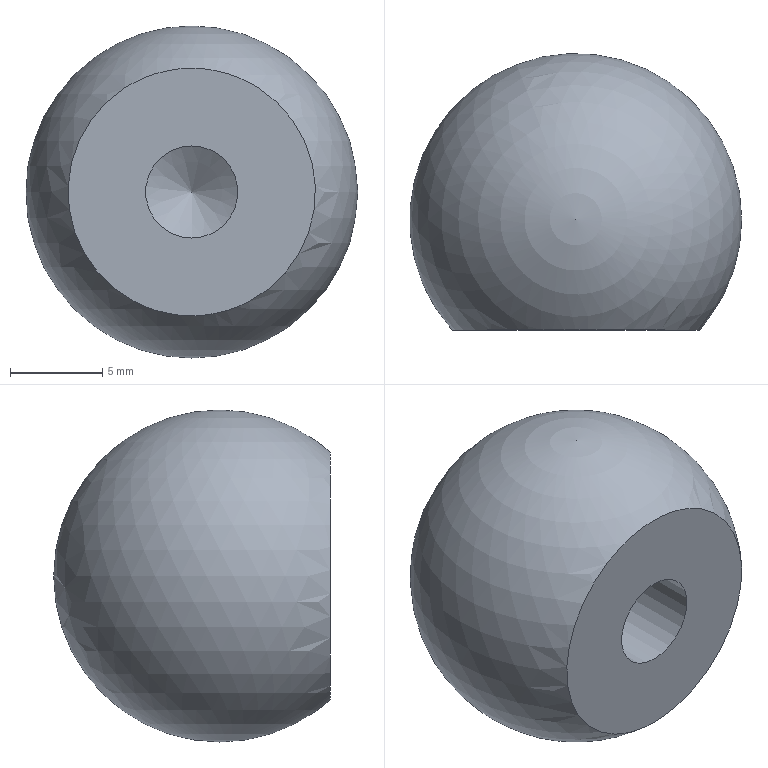Part | NX | features ABSOLUTE_DATUM_PLANE 1, DATUM_CSYS 1, HOLE PACKAGE 1, SIMPLE HOLE 1, SPHERE 1, SYMBOLIC_THREAD 1, TRIM BODY 1 | 1 solid | 4 faces | box 18 x 15 x 18 mm | volume 2621 mm3 | sphere 1 | plane 1 | cone 1 | cylinder 1 | commonest cylinder face diameters 5 x1
STEP:
#1=CARTESIAN_POINT('',(0.,-6.,6.708));
#2=VERTEX_POINT('',#1);
#3=CARTESIAN_POINT('',(0.,-6.,0.));
#4=DIRECTION('',(0.,1.,0.));
#5=DIRECTION('',(0.,0.,1.));
#6=AXIS2_PLACEMENT_3D('',#3,#4,#5);
#7=CIRCLE('',#6,6.708);
#8=EDGE_CURVE('',#2,#2,#7,.F.);
#9=ORIENTED_EDGE('',*,*,#8,.F.);
#10=EDGE_LOOP('',(#9));
#11=FACE_BOUND('',#10,.T.);
#12=CARTESIAN_POINT('',(0.,0.,0.));
#13=DIRECTION('',(0.,0.,1.));
#14=DIRECTION('',(1.,0.,0.));
#15=AXIS2_PLACEMENT_3D('',#12,#13,#14);
#16=SPHERICAL_SURFACE('',#15,9.);
#17=ADVANCED_FACE('',(#11),#16,.T.);
#18=CARTESIAN_POINT('',(0.,-6.,2.5));
#19=VERTEX_POINT('',#18);
#20=CARTESIAN_POINT('',(0.,-6.,0.));
#21=DIRECTION('',(0.,1.,0.));
#22=DIRECTION('',(0.,0.,1.));
#23=AXIS2_PLACEMENT_3D('',#20,#21,#22);
#24=CIRCLE('',#23,2.5);
#25=EDGE_CURVE('',#19,#19,#24,.T.);
#26=ORIENTED_EDGE('',*,*,#25,.T.);
#27=EDGE_LOOP('',(#26));
#28=FACE_BOUND('',#27,.T.);
#29=ORIENTED_EDGE('',*,*,#8,.T.);
#30=EDGE_LOOP('',(#29));
#31=FACE_BOUND('',#30,.T.);
#32=CARTESIAN_POINT('',(0.,-6.,0.));
#33=DIRECTION('',(0.,1.,0.));
#34=DIRECTION('',(0.,0.,1.));
#35=AXIS2_PLACEMENT_3D('',#32,#33,#34);
#36=PLANE('',#35);
#37=ADVANCED_FACE('',(#28,#31),#36,.F.);
#38=CARTESIAN_POINT('',(0.,4.,2.5));
#39=VERTEX_POINT('',#38);
#40=CARTESIAN_POINT('',(0.,4.,0.));
#41=DIRECTION('',(0.,1.,0.));
#42=DIRECTION('',(0.,0.,1.));
#43=AXIS2_PLACEMENT_3D('',#40,#41,#42);
#44=CIRCLE('',#43,2.5);
#45=EDGE_CURVE('',#39,#39,#44,.F.);
#46=ORIENTED_EDGE('',*,*,#45,.T.);
#47=EDGE_LOOP('',(#46));
#48=FACE_BOUND('',#47,.T.);
#49=CARTESIAN_POINT('',(0.,5.502,0.));
#50=VERTEX_POINT('',#49);
#51=VERTEX_LOOP('',#50);
#52=FACE_BOUND('',#51,.T.);
#53=CARTESIAN_POINT('',(0.,4.,0.));
#54=DIRECTION('',(0.,-1.,0.));
#55=DIRECTION('',(0.,0.,-1.));
#56=AXIS2_PLACEMENT_3D('',#53,#54,#55);
#57=CONICAL_SURFACE('',#56,2.5,1.03);
#58=ADVANCED_FACE('',(#48,#52),#57,.F.);
#59=ORIENTED_EDGE('',*,*,#45,.F.);
#60=EDGE_LOOP('',(#59));
#61=FACE_BOUND('',#60,.T.);
#62=ORIENTED_EDGE('',*,*,#25,.F.);
#63=EDGE_LOOP('',(#62));
#64=FACE_BOUND('',#63,.T.);
#65=CARTESIAN_POINT('',(0.,-6.,0.));
#66=DIRECTION('',(0.,1.,0.));
#67=DIRECTION('',(0.,0.,1.));
#68=AXIS2_PLACEMENT_3D('',#65,#66,#67);
#69=CYLINDRICAL_SURFACE('',#68,2.5);
#70=ADVANCED_FACE('',(#61,#64),#69,.F.);
#71=CLOSED_SHELL('',(#17,#37,#58,#70));
#72=MANIFOLD_SOLID_BREP('',#71);
#73=(LENGTH_UNIT()NAMED_UNIT(*)SI_UNIT(.MILLI.,.METRE.));
#74=UNCERTAINTY_MEASURE_WITH_UNIT(LENGTH_MEASURE(0.00001),#73,'','');
#75=(NAMED_UNIT(*)PLANE_ANGLE_UNIT()SI_UNIT($,.RADIAN.));
#76=(NAMED_UNIT(*)SI_UNIT($,.STERADIAN.)SOLID_ANGLE_UNIT());
#77=(GEOMETRIC_REPRESENTATION_CONTEXT(3)GLOBAL_UNCERTAINTY_ASSIGNED_CONTEXT((#74))GLOBAL_UNIT_ASSIGNED_CONTEXT((#73,#75,#76))REPRESENTATION_CONTEXT('',''));
#78=ADVANCED_BREP_SHAPE_REPRESENTATION('',(#72),#77);